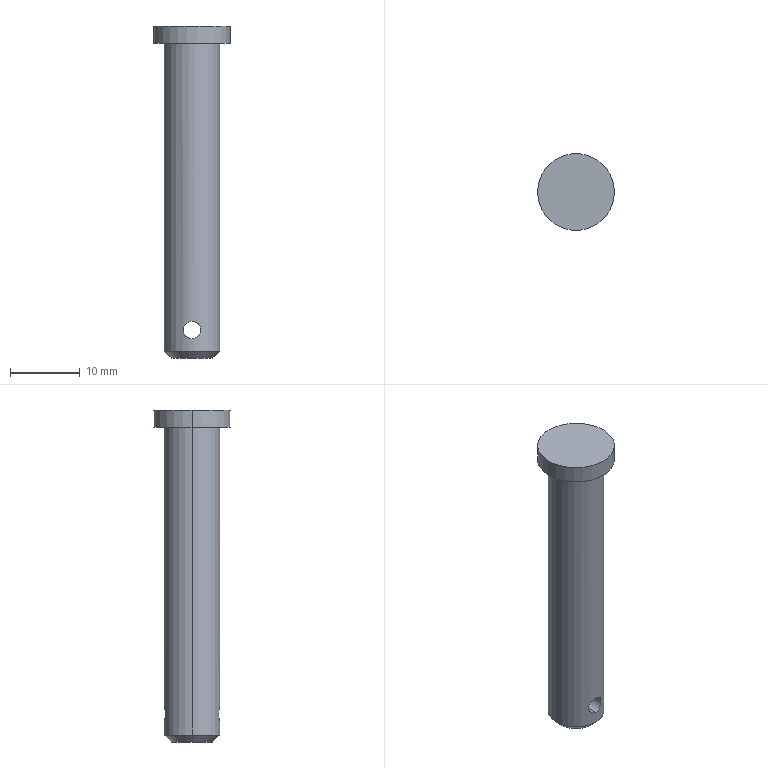Part | NX | features BREP 1 | 1 solid | 11 faces | box 11 x 11 x 47.5 mm | volume 2449 mm3 | cylinder 6 | plane 3 | cone 2 | commonest cylinder face diameters 2.5 x2 8 x2 11 x2
STEP:
#1=CARTESIAN_POINT('',(3.,0.,0.));
#2=VERTEX_POINT('',#1);
#3=CARTESIAN_POINT('',(-3.,0.,0.));
#4=VERTEX_POINT('',#3);
#5=CARTESIAN_POINT('',(0.,0.,0.));
#6=DIRECTION('',(0.,0.,-1.));
#7=DIRECTION('',(1.,0.,0.));
#8=AXIS2_PLACEMENT_3D('',#5,#6,#7);
#9=CIRCLE('',#8,3.);
#10=EDGE_CURVE('',#2,#4,#9,.T.);
#11=ORIENTED_EDGE('',*,*,#10,.F.);
#12=CARTESIAN_POINT('',(4.,0.,1.));
#13=VERTEX_POINT('',#12);
#14=CARTESIAN_POINT('',(4.,0.,1.));
#15=DIRECTION('',(-0.7071,0.,-0.7071));
#16=VECTOR('',#15,1000.);
#17=LINE('',#14,#16);
#18=EDGE_CURVE('',#13,#2,#17,.T.);
#19=ORIENTED_EDGE('',*,*,#18,.F.);
#20=CARTESIAN_POINT('',(-4.,0.,1.));
#21=VERTEX_POINT('',#20);
#22=CARTESIAN_POINT('',(0.,0.,1.));
#23=DIRECTION('',(0.,0.,-1.));
#24=DIRECTION('',(1.,0.,0.));
#25=AXIS2_PLACEMENT_3D('',#22,#23,#24);
#26=CIRCLE('',#25,4.);
#27=EDGE_CURVE('',#13,#21,#26,.T.);
#28=ORIENTED_EDGE('',*,*,#27,.T.);
#29=CARTESIAN_POINT('',(-4.,0.,1.));
#30=DIRECTION('',(0.7071,0.,-0.7071));
#31=VECTOR('',#30,1000.);
#32=LINE('',#29,#31);
#33=EDGE_CURVE('',#21,#4,#32,.T.);
#34=ORIENTED_EDGE('',*,*,#33,.T.);
#35=EDGE_LOOP('',(#11,#19,#28,#34));
#36=FACE_BOUND('',#35,.T.);
#37=CARTESIAN_POINT('',(0.,0.,0.5));
#38=DIRECTION('',(0.,0.,1.));
#39=DIRECTION('',(-1.,0.,0.));
#40=AXIS2_PLACEMENT_3D('',#37,#38,#39);
#41=CONICAL_SURFACE('',#40,3.5,0.7854);
#42=ADVANCED_FACE('',(#36),#41,.T.);
#43=ORIENTED_EDGE('',*,*,#33,.F.);
#44=CARTESIAN_POINT('',(0.,0.,1.));
#45=DIRECTION('',(0.,0.,-1.));
#46=DIRECTION('',(-1.,0.,0.));
#47=AXIS2_PLACEMENT_3D('',#44,#45,#46);
#48=CIRCLE('',#47,4.);
#49=EDGE_CURVE('',#21,#13,#48,.T.);
#50=ORIENTED_EDGE('',*,*,#49,.T.);
#51=ORIENTED_EDGE('',*,*,#18,.T.);
#52=CARTESIAN_POINT('',(0.,0.,0.));
#53=DIRECTION('',(0.,0.,-1.));
#54=DIRECTION('',(-1.,0.,0.));
#55=AXIS2_PLACEMENT_3D('',#52,#53,#54);
#56=CIRCLE('',#55,3.);
#57=EDGE_CURVE('',#4,#2,#56,.T.);
#58=ORIENTED_EDGE('',*,*,#57,.F.);
#59=EDGE_LOOP('',(#43,#50,#51,#58));
#60=FACE_BOUND('',#59,.T.);
#61=CARTESIAN_POINT('',(0.,0.,0.5));
#62=DIRECTION('',(0.,0.,1.));
#63=DIRECTION('',(-1.,0.,0.));
#64=AXIS2_PLACEMENT_3D('',#61,#62,#63);
#65=CONICAL_SURFACE('',#64,3.5,0.7854);
#66=ADVANCED_FACE('',(#60),#65,.T.);
#67=ORIENTED_EDGE('',*,*,#57,.T.);
#68=ORIENTED_EDGE('',*,*,#10,.T.);
#69=EDGE_LOOP('',(#67,#68));
#70=FACE_BOUND('',#69,.T.);
#71=CARTESIAN_POINT('',(0.,0.,0.));
#72=DIRECTION('',(0.,0.,1.));
#73=DIRECTION('',(-1.,0.,0.));
#74=AXIS2_PLACEMENT_3D('',#71,#72,#73);
#75=PLANE('',#74);
#76=ADVANCED_FACE('',(#70),#75,.F.);
#77=CARTESIAN_POINT('',(4.,0.,45.));
#78=VERTEX_POINT('',#77);
#79=CARTESIAN_POINT('',(4.,0.,1.));
#80=DIRECTION('',(0.,0.,1.));
#81=VECTOR('',#80,1000.);
#82=LINE('',#79,#81);
#83=EDGE_CURVE('',#13,#78,#82,.T.);
#84=ORIENTED_EDGE('',*,*,#83,.F.);
#85=ORIENTED_EDGE('',*,*,#49,.F.);
#86=CARTESIAN_POINT('',(-4.,0.,45.));
#87=VERTEX_POINT('',#86);
#88=CARTESIAN_POINT('',(-4.,0.,1.));
#89=DIRECTION('',(0.,0.,1.));
#90=VECTOR('',#89,1000.);
#91=LINE('',#88,#90);
#92=EDGE_CURVE('',#21,#87,#91,.T.);
#93=ORIENTED_EDGE('',*,*,#92,.T.);
#94=CARTESIAN_POINT('',(0.,0.,45.));
#95=DIRECTION('',(0.,0.,1.));
#96=DIRECTION('',(1.,0.,0.));
#97=AXIS2_PLACEMENT_3D('',#94,#95,#96);
#98=CIRCLE('',#97,4.);
#99=EDGE_CURVE('',#78,#87,#98,.T.);
#100=ORIENTED_EDGE('',*,*,#99,.F.);
#101=EDGE_LOOP('',(#84,#85,#93,#100));
#102=FACE_BOUND('',#101,.T.);
#103=CARTESIAN_POINT('',(0.,4.,5.25));
#104=VERTEX_POINT('',#103);
#105=CARTESIAN_POINT('',(0.,4.,2.75));
#106=VERTEX_POINT('',#105);
#107=CARTESIAN_POINT('',(0.,4.,5.25));
#108=CARTESIAN_POINT('',(0.3325,4.,5.25));
#109=CARTESIAN_POINT('',(0.9768,3.902,4.979));
#110=CARTESIAN_POINT('',(1.386,3.748,4.002));
#111=CARTESIAN_POINT('',(0.9773,3.902,3.021));
#112=CARTESIAN_POINT('',(0.3325,4.,2.75));
#113=CARTESIAN_POINT('',(0.,4.,2.75));
#114=B_SPLINE_CURVE_WITH_KNOTS('',3,(#107,#108,#109,#110,#111,#112,#113),.UNSPECIFIED.,.F.,.F.,(4,1,1,1,4),(0.,0.0009829,0.001966,0.002949,0.003931),.UNSPECIFIED.);
#115=EDGE_CURVE('',#104,#106,#114,.T.);
#116=ORIENTED_EDGE('',*,*,#115,.F.);
#117=CARTESIAN_POINT('',(0.,4.,2.75));
#118=CARTESIAN_POINT('',(-0.3325,4.,2.75));
#119=CARTESIAN_POINT('',(-0.9768,3.902,3.021));
#120=CARTESIAN_POINT('',(-1.386,3.748,3.998));
#121=CARTESIAN_POINT('',(-0.9773,3.902,4.979));
#122=CARTESIAN_POINT('',(-0.3325,4.,5.25));
#123=CARTESIAN_POINT('',(0.,4.,5.25));
#124=B_SPLINE_CURVE_WITH_KNOTS('',3,(#117,#118,#119,#120,#121,#122,#123),.UNSPECIFIED.,.F.,.F.,(4,1,1,1,4),(0.,0.0009829,0.001966,0.002949,0.003931),.UNSPECIFIED.);
#125=EDGE_CURVE('',#106,#104,#124,.T.);
#126=ORIENTED_EDGE('',*,*,#125,.F.);
#127=EDGE_LOOP('',(#116,#126));
#128=FACE_BOUND('',#127,.T.);
#129=CARTESIAN_POINT('',(0.,0.,45.));
#130=DIRECTION('',(0.,0.,-1.));
#131=DIRECTION('',(1.,0.,0.));
#132=AXIS2_PLACEMENT_3D('',#129,#130,#131);
#133=CYLINDRICAL_SURFACE('',#132,4.);
#134=ADVANCED_FACE('',(#102,#128),#133,.T.);
#135=CARTESIAN_POINT('',(-5.5,0.,45.));
#136=VERTEX_POINT('',#135);
#137=CARTESIAN_POINT('',(5.5,0.,45.));
#138=VERTEX_POINT('',#137);
#139=CARTESIAN_POINT('',(0.,0.,45.));
#140=DIRECTION('',(0.,0.,-1.));
#141=DIRECTION('',(-1.,0.,0.));
#142=AXIS2_PLACEMENT_3D('',#139,#140,#141);
#143=CIRCLE('',#142,5.5);
#144=EDGE_CURVE('',#136,#138,#143,.T.);
#145=ORIENTED_EDGE('',*,*,#144,.T.);
#146=CARTESIAN_POINT('',(0.,0.,45.));
#147=DIRECTION('',(0.,0.,-1.));
#148=DIRECTION('',(1.,0.,0.));
#149=AXIS2_PLACEMENT_3D('',#146,#147,#148);
#150=CIRCLE('',#149,5.5);
#151=EDGE_CURVE('',#138,#136,#150,.T.);
#152=ORIENTED_EDGE('',*,*,#151,.T.);
#153=EDGE_LOOP('',(#145,#152));
#154=FACE_BOUND('',#153,.T.);
#155=ORIENTED_EDGE('',*,*,#99,.T.);
#156=CARTESIAN_POINT('',(0.,0.,45.));
#157=DIRECTION('',(0.,0.,1.));
#158=DIRECTION('',(-1.,0.,0.));
#159=AXIS2_PLACEMENT_3D('',#156,#157,#158);
#160=CIRCLE('',#159,4.);
#161=EDGE_CURVE('',#87,#78,#160,.T.);
#162=ORIENTED_EDGE('',*,*,#161,.T.);
#163=EDGE_LOOP('',(#155,#162));
#164=FACE_BOUND('',#163,.T.);
#165=CARTESIAN_POINT('',(0.,0.,45.));
#166=DIRECTION('',(0.,0.,1.));
#167=DIRECTION('',(-1.,0.,0.));
#168=AXIS2_PLACEMENT_3D('',#165,#166,#167);
#169=PLANE('',#168);
#170=ADVANCED_FACE('',(#154,#164),#169,.F.);
#171=CARTESIAN_POINT('',(-5.5,0.,47.5));
#172=VERTEX_POINT('',#171);
#173=CARTESIAN_POINT('',(5.5,0.,47.5));
#174=VERTEX_POINT('',#173);
#175=CARTESIAN_POINT('',(0.,0.,47.5));
#176=DIRECTION('',(0.,0.,1.));
#177=DIRECTION('',(-1.,0.,0.));
#178=AXIS2_PLACEMENT_3D('',#175,#176,#177);
#179=CIRCLE('',#178,5.5);
#180=EDGE_CURVE('',#172,#174,#179,.T.);
#181=ORIENTED_EDGE('',*,*,#180,.F.);
#182=CARTESIAN_POINT('',(-5.5,0.,45.));
#183=DIRECTION('',(0.,0.,1.));
#184=VECTOR('',#183,1000.);
#185=LINE('',#182,#184);
#186=EDGE_CURVE('',#172,#136,#185,.F.);
#187=ORIENTED_EDGE('',*,*,#186,.T.);
#188=ORIENTED_EDGE('',*,*,#151,.F.);
#189=CARTESIAN_POINT('',(5.5,0.,45.));
#190=DIRECTION('',(0.,0.,1.));
#191=VECTOR('',#190,1000.);
#192=LINE('',#189,#191);
#193=EDGE_CURVE('',#174,#138,#192,.F.);
#194=ORIENTED_EDGE('',*,*,#193,.F.);
#195=EDGE_LOOP('',(#181,#187,#188,#194));
#196=FACE_BOUND('',#195,.T.);
#197=CARTESIAN_POINT('',(0.,0.,47.5));
#198=DIRECTION('',(0.,0.,-1.));
#199=DIRECTION('',(1.,0.,0.));
#200=AXIS2_PLACEMENT_3D('',#197,#198,#199);
#201=CYLINDRICAL_SURFACE('',#200,5.5);
#202=ADVANCED_FACE('',(#196),#201,.T.);
#203=ORIENTED_EDGE('',*,*,#193,.T.);
#204=ORIENTED_EDGE('',*,*,#144,.F.);
#205=ORIENTED_EDGE('',*,*,#186,.F.);
#206=CARTESIAN_POINT('',(0.,0.,47.5));
#207=DIRECTION('',(0.,0.,1.));
#208=DIRECTION('',(1.,0.,0.));
#209=AXIS2_PLACEMENT_3D('',#206,#207,#208);
#210=CIRCLE('',#209,5.5);
#211=EDGE_CURVE('',#174,#172,#210,.T.);
#212=ORIENTED_EDGE('',*,*,#211,.F.);
#213=EDGE_LOOP('',(#203,#204,#205,#212));
#214=FACE_BOUND('',#213,.T.);
#215=CARTESIAN_POINT('',(0.,0.,47.5));
#216=DIRECTION('',(0.,0.,-1.));
#217=DIRECTION('',(1.,0.,0.));
#218=AXIS2_PLACEMENT_3D('',#215,#216,#217);
#219=CYLINDRICAL_SURFACE('',#218,5.5);
#220=ADVANCED_FACE('',(#214),#219,.T.);
#221=ORIENTED_EDGE('',*,*,#211,.T.);
#222=ORIENTED_EDGE('',*,*,#180,.T.);
#223=EDGE_LOOP('',(#221,#222));
#224=FACE_BOUND('',#223,.T.);
#225=CARTESIAN_POINT('',(0.,0.,47.5));
#226=DIRECTION('',(0.,0.,1.));
#227=DIRECTION('',(-1.,0.,0.));
#228=AXIS2_PLACEMENT_3D('',#225,#226,#227);
#229=PLANE('',#228);
#230=ADVANCED_FACE('',(#224),#229,.T.);
#231=ORIENTED_EDGE('',*,*,#161,.F.);
#232=ORIENTED_EDGE('',*,*,#92,.F.);
#233=ORIENTED_EDGE('',*,*,#27,.F.);
#234=ORIENTED_EDGE('',*,*,#83,.T.);
#235=EDGE_LOOP('',(#231,#232,#233,#234));
#236=FACE_BOUND('',#235,.T.);
#237=CARTESIAN_POINT('',(0.,-4.,5.25));
#238=VERTEX_POINT('',#237);
#239=CARTESIAN_POINT('',(0.,-4.,2.75));
#240=VERTEX_POINT('',#239);
#241=CARTESIAN_POINT('',(0.,-4.,5.25));
#242=CARTESIAN_POINT('',(-0.3325,-4.,5.25));
#243=CARTESIAN_POINT('',(-0.9768,-3.902,4.979));
#244=CARTESIAN_POINT('',(-1.386,-3.748,4.002));
#245=CARTESIAN_POINT('',(-0.9773,-3.902,3.021));
#246=CARTESIAN_POINT('',(-0.3325,-4.,2.75));
#247=CARTESIAN_POINT('',(0.,-4.,2.75));
#248=B_SPLINE_CURVE_WITH_KNOTS('',3,(#241,#242,#243,#244,#245,#246,#247),.UNSPECIFIED.,.F.,.F.,(4,1,1,1,4),(0.,0.0009829,0.001966,0.002949,0.003931),.UNSPECIFIED.);
#249=EDGE_CURVE('',#238,#240,#248,.T.);
#250=ORIENTED_EDGE('',*,*,#249,.F.);
#251=CARTESIAN_POINT('',(0.,-4.,2.75));
#252=CARTESIAN_POINT('',(0.3325,-4.,2.75));
#253=CARTESIAN_POINT('',(0.9768,-3.902,3.021));
#254=CARTESIAN_POINT('',(1.386,-3.748,3.998));
#255=CARTESIAN_POINT('',(0.9773,-3.902,4.979));
#256=CARTESIAN_POINT('',(0.3325,-4.,5.25));
#257=CARTESIAN_POINT('',(0.,-4.,5.25));
#258=B_SPLINE_CURVE_WITH_KNOTS('',3,(#251,#252,#253,#254,#255,#256,#257),.UNSPECIFIED.,.F.,.F.,(4,1,1,1,4),(0.,0.0009829,0.001966,0.002949,0.003931),.UNSPECIFIED.);
#259=EDGE_CURVE('',#240,#238,#258,.T.);
#260=ORIENTED_EDGE('',*,*,#259,.F.);
#261=EDGE_LOOP('',(#250,#260));
#262=FACE_BOUND('',#261,.T.);
#263=CARTESIAN_POINT('',(0.,0.,45.));
#264=DIRECTION('',(0.,0.,-1.));
#265=DIRECTION('',(1.,0.,0.));
#266=AXIS2_PLACEMENT_3D('',#263,#264,#265);
#267=CYLINDRICAL_SURFACE('',#266,4.);
#268=ADVANCED_FACE('',(#236,#262),#267,.T.);
#269=ORIENTED_EDGE('',*,*,#259,.T.);
#270=CARTESIAN_POINT('',(0.,4.,5.25));
#271=DIRECTION('',(0.,-1.,0.));
#272=VECTOR('',#271,1000.);
#273=LINE('',#270,#272);
#274=EDGE_CURVE('',#104,#238,#273,.T.);
#275=ORIENTED_EDGE('',*,*,#274,.F.);
#276=ORIENTED_EDGE('',*,*,#115,.T.);
#277=CARTESIAN_POINT('',(0.,4.,2.75));
#278=DIRECTION('',(0.,-1.,0.));
#279=VECTOR('',#278,1000.);
#280=LINE('',#277,#279);
#281=EDGE_CURVE('',#106,#240,#280,.T.);
#282=ORIENTED_EDGE('',*,*,#281,.T.);
#283=EDGE_LOOP('',(#269,#275,#276,#282));
#284=FACE_BOUND('',#283,.T.);
#285=CARTESIAN_POINT('',(0.,-6.25,4.));
#286=DIRECTION('',(0.,1.,0.));
#287=DIRECTION('',(0.,0.,-1.));
#288=AXIS2_PLACEMENT_3D('',#285,#286,#287);
#289=CYLINDRICAL_SURFACE('',#288,1.25);
#290=ADVANCED_FACE('',(#284),#289,.F.);
#291=ORIENTED_EDGE('',*,*,#281,.F.);
#292=ORIENTED_EDGE('',*,*,#125,.T.);
#293=ORIENTED_EDGE('',*,*,#274,.T.);
#294=ORIENTED_EDGE('',*,*,#249,.T.);
#295=EDGE_LOOP('',(#291,#292,#293,#294));
#296=FACE_BOUND('',#295,.T.);
#297=CARTESIAN_POINT('',(0.,-6.25,4.));
#298=DIRECTION('',(0.,1.,0.));
#299=DIRECTION('',(0.,0.,-1.));
#300=AXIS2_PLACEMENT_3D('',#297,#298,#299);
#301=CYLINDRICAL_SURFACE('',#300,1.25);
#302=ADVANCED_FACE('',(#296),#301,.F.);
#303=CLOSED_SHELL('',(#42,#66,#76,#134,#170,#202,#220,#230,#268,#290,#302));
#304=MANIFOLD_SOLID_BREP('',#303);
#305=(LENGTH_UNIT()NAMED_UNIT(*)SI_UNIT(.MILLI.,.METRE.));
#306=UNCERTAINTY_MEASURE_WITH_UNIT(LENGTH_MEASURE(0.0508),#305,'','');
#307=(NAMED_UNIT(*)PLANE_ANGLE_UNIT()SI_UNIT($,.RADIAN.));
#308=(NAMED_UNIT(*)SI_UNIT($,.STERADIAN.)SOLID_ANGLE_UNIT());
#309=(GEOMETRIC_REPRESENTATION_CONTEXT(3)GLOBAL_UNCERTAINTY_ASSIGNED_CONTEXT((#306))GLOBAL_UNIT_ASSIGNED_CONTEXT((#305,#307,#308))REPRESENTATION_CONTEXT('',''));
#310=ADVANCED_BREP_SHAPE_REPRESENTATION('',(#304),#309);